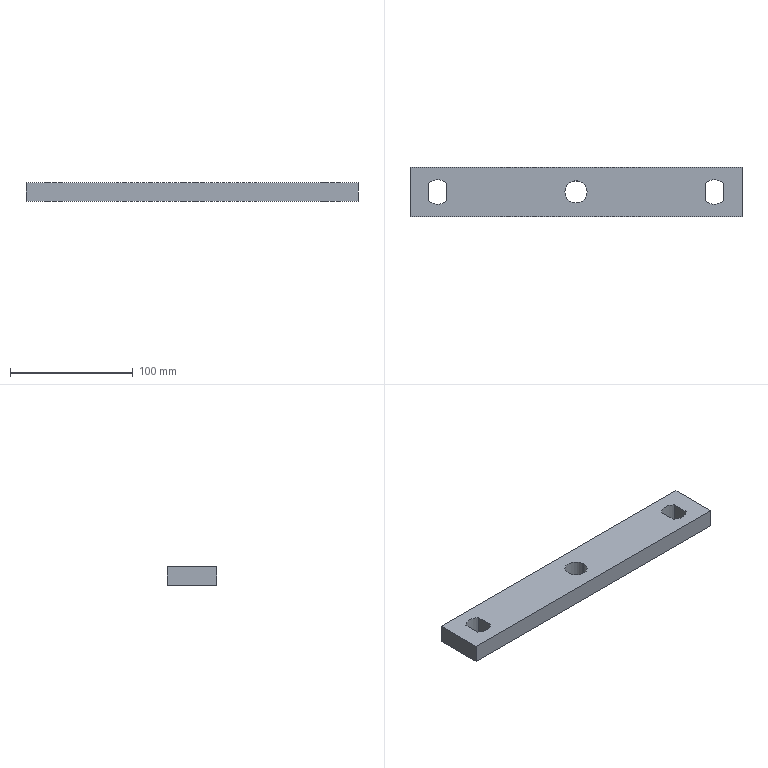Part | STEP file | Link hanger plate | 1 solid | 16 faces | box 270 x 40 x 15 mm | volume 150118 mm3 | plane 10 | cylinder 6 | commonest cylinder face diameters 20 x4 18 x2
STEP:
#1=CARTESIAN_POINT('',(0.,0.,0.));
#2=DIRECTION('',(0.,0.,1.));
#3=DIRECTION('',(1.,0.,0.));
#4=AXIS2_PLACEMENT_3D('',#1,#2,#3);
#5=CARTESIAN_POINT('',(9.,10.,-7.5));
#6=VERTEX_POINT('',#5);
#7=CARTESIAN_POINT('',(9.,10.,7.5));
#8=VERTEX_POINT('',#7);
#9=CARTESIAN_POINT('',(9.,10.,7.5));
#10=DIRECTION('',(0.,0.,1.));
#11=VECTOR('',#10,1.);
#12=LINE('',#9,#11);
#13=CARTESIAN_POINT('',(0.,10.,7.5));
#14=DIRECTION('',(0.,0.,1.));
#15=DIRECTION('',(1.,0.,0.));
#16=AXIS2_PLACEMENT_3D('',#13,#14,#15);
#17=CYLINDRICAL_SURFACE('',#16,9.);
#18=CARTESIAN_POINT('',(6.283,0.));
#19=DIRECTION('',(0.,1.));
#20=VECTOR('',#19,1.);
#21=LINE('',#18,#20);
#22=(GEOMETRIC_REPRESENTATION_CONTEXT(2)PARAMETRIC_REPRESENTATION_CONTEXT()REPRESENTATION_CONTEXT('',''));
#23=DEFINITIONAL_REPRESENTATION('',(#21),#22);
#24=PCURVE('',#17,#23);
#25=CARTESIAN_POINT('',(0.,10.,7.5));
#26=DIRECTION('',(0.,0.,1.));
#27=DIRECTION('',(1.,0.,0.));
#28=AXIS2_PLACEMENT_3D('',#25,#26,#27);
#29=CYLINDRICAL_SURFACE('',#28,9.);
#30=CARTESIAN_POINT('',(0.,0.));
#31=DIRECTION('',(0.,1.));
#32=VECTOR('',#31,1.);
#33=LINE('',#30,#32);
#34=(GEOMETRIC_REPRESENTATION_CONTEXT(2)PARAMETRIC_REPRESENTATION_CONTEXT()REPRESENTATION_CONTEXT('',''));
#35=DEFINITIONAL_REPRESENTATION('',(#33),#34);
#36=PCURVE('',#29,#35);
#37=SURFACE_CURVE('',#12,(#24,#36),.PCURVE_S1.);
#38=EDGE_CURVE('',#6,#8,#37,.T.);
#39=ORIENTED_EDGE('',*,*,#38,.T.);
#40=CARTESIAN_POINT('',(-9.,10.,7.5));
#41=VERTEX_POINT('',#40);
#42=CARTESIAN_POINT('',(0.,10.,7.5));
#43=DIRECTION('',(0.,0.,1.));
#44=DIRECTION('',(1.,0.,0.));
#45=AXIS2_PLACEMENT_3D('',#42,#43,#44);
#46=CIRCLE('',#45,9.);
#47=CARTESIAN_POINT('',(0.,0.));
#48=DIRECTION('',(1.,0.));
#49=VECTOR('',#48,1.);
#50=LINE('',#47,#49);
#51=(GEOMETRIC_REPRESENTATION_CONTEXT(2)PARAMETRIC_REPRESENTATION_CONTEXT()REPRESENTATION_CONTEXT('',''));
#52=DEFINITIONAL_REPRESENTATION('',(#50),#51);
#53=PCURVE('',#17,#52);
#54=CARTESIAN_POINT('',(0.,0.,7.5));
#55=DIRECTION('',(0.,0.,1.));
#56=DIRECTION('',(1.,0.,0.));
#57=AXIS2_PLACEMENT_3D('',#54,#55,#56);
#58=PLANE('',#57);
#59=CARTESIAN_POINT('',(0.,10.));
#60=DIRECTION('',(1.,0.));
#61=AXIS2_PLACEMENT_2D('',#59,#60);
#62=CIRCLE('',#61,9.);
#63=(GEOMETRIC_REPRESENTATION_CONTEXT(2)PARAMETRIC_REPRESENTATION_CONTEXT()REPRESENTATION_CONTEXT('',''));
#64=DEFINITIONAL_REPRESENTATION('',(#62),#63);
#65=PCURVE('',#58,#64);
#66=SURFACE_CURVE('',#46,(#53,#65),.PCURVE_S1.);
#67=EDGE_CURVE('',#41,#8,#66,.T.);
#68=ORIENTED_EDGE('',*,*,#67,.F.);
#69=CARTESIAN_POINT('',(-9.,10.,-7.5));
#70=VERTEX_POINT('',#69);
#71=CARTESIAN_POINT('',(-9.,10.,7.5));
#72=DIRECTION('',(0.,0.,1.));
#73=VECTOR('',#72,1.);
#74=LINE('',#71,#73);
#75=CARTESIAN_POINT('',(3.142,0.));
#76=DIRECTION('',(0.,1.));
#77=VECTOR('',#76,1.);
#78=LINE('',#75,#77);
#79=(GEOMETRIC_REPRESENTATION_CONTEXT(2)PARAMETRIC_REPRESENTATION_CONTEXT()REPRESENTATION_CONTEXT('',''));
#80=DEFINITIONAL_REPRESENTATION('',(#78),#79);
#81=PCURVE('',#17,#80);
#82=CARTESIAN_POINT('',(3.142,0.));
#83=DIRECTION('',(0.,1.));
#84=VECTOR('',#83,1.);
#85=LINE('',#82,#84);
#86=(GEOMETRIC_REPRESENTATION_CONTEXT(2)PARAMETRIC_REPRESENTATION_CONTEXT()REPRESENTATION_CONTEXT('',''));
#87=DEFINITIONAL_REPRESENTATION('',(#85),#86);
#88=PCURVE('',#29,#87);
#89=SURFACE_CURVE('',#74,(#81,#88),.PCURVE_S1.);
#90=EDGE_CURVE('',#70,#41,#89,.T.);
#91=ORIENTED_EDGE('',*,*,#90,.F.);
#92=CARTESIAN_POINT('',(0.,10.,-7.5));
#93=DIRECTION('',(0.,0.,1.));
#94=DIRECTION('',(1.,0.,0.));
#95=AXIS2_PLACEMENT_3D('',#92,#93,#94);
#96=CIRCLE('',#95,9.);
#97=CARTESIAN_POINT('',(0.,-15.));
#98=DIRECTION('',(1.,0.));
#99=VECTOR('',#98,1.);
#100=LINE('',#97,#99);
#101=(GEOMETRIC_REPRESENTATION_CONTEXT(2)PARAMETRIC_REPRESENTATION_CONTEXT()REPRESENTATION_CONTEXT('',''));
#102=DEFINITIONAL_REPRESENTATION('',(#100),#101);
#103=PCURVE('',#17,#102);
#104=CARTESIAN_POINT('',(0.,0.,-7.5));
#105=DIRECTION('',(0.,0.,1.));
#106=DIRECTION('',(1.,0.,0.));
#107=AXIS2_PLACEMENT_3D('',#104,#105,#106);
#108=PLANE('',#107);
#109=CARTESIAN_POINT('',(0.,10.));
#110=DIRECTION('',(1.,0.));
#111=AXIS2_PLACEMENT_2D('',#109,#110);
#112=CIRCLE('',#111,9.);
#113=(GEOMETRIC_REPRESENTATION_CONTEXT(2)PARAMETRIC_REPRESENTATION_CONTEXT()REPRESENTATION_CONTEXT('',''));
#114=DEFINITIONAL_REPRESENTATION('',(#112),#113);
#115=PCURVE('',#108,#114);
#116=SURFACE_CURVE('',#96,(#103,#115),.PCURVE_S1.);
#117=EDGE_CURVE('',#70,#6,#116,.T.);
#118=ORIENTED_EDGE('',*,*,#117,.T.);
#119=EDGE_LOOP('',(#39,#68,#91,#118));
#120=FACE_BOUND('',#119,.F.);
#121=ADVANCED_FACE('',(#120),#17,.F.);
#122=CARTESIAN_POINT('',(-135.,30.,7.5));
#123=VERTEX_POINT('',#122);
#124=CARTESIAN_POINT('',(-135.,-10.,7.5));
#125=VERTEX_POINT('',#124);
#126=CARTESIAN_POINT('',(-135.,30.,7.5));
#127=DIRECTION('',(0.,-1.,0.));
#128=VECTOR('',#127,1.);
#129=LINE('',#126,#128);
#130=CARTESIAN_POINT('',(-135.,30.));
#131=DIRECTION('',(0.,-1.));
#132=VECTOR('',#131,1.);
#133=LINE('',#130,#132);
#134=(GEOMETRIC_REPRESENTATION_CONTEXT(2)PARAMETRIC_REPRESENTATION_CONTEXT()REPRESENTATION_CONTEXT('',''));
#135=DEFINITIONAL_REPRESENTATION('',(#133),#134);
#136=PCURVE('',#58,#135);
#137=CARTESIAN_POINT('',(-135.,30.,7.5));
#138=DIRECTION('',(1.,0.,0.));
#139=DIRECTION('',(0.,0.,-1.));
#140=AXIS2_PLACEMENT_3D('',#137,#138,#139);
#141=PLANE('',#140);
#142=CARTESIAN_POINT('',(0.,0.));
#143=DIRECTION('',(0.,-1.));
#144=VECTOR('',#143,1.);
#145=LINE('',#142,#144);
#146=(GEOMETRIC_REPRESENTATION_CONTEXT(2)PARAMETRIC_REPRESENTATION_CONTEXT()REPRESENTATION_CONTEXT('',''));
#147=DEFINITIONAL_REPRESENTATION('',(#145),#146);
#148=PCURVE('',#141,#147);
#149=SURFACE_CURVE('',#129,(#136,#148),.PCURVE_S1.);
#150=EDGE_CURVE('',#123,#125,#149,.T.);
#151=ORIENTED_EDGE('',*,*,#150,.T.);
#152=CARTESIAN_POINT('',(135.,-10.,7.5));
#153=VERTEX_POINT('',#152);
#154=CARTESIAN_POINT('',(135.,-10.,7.5));
#155=DIRECTION('',(1.,0.,0.));
#156=VECTOR('',#155,1.);
#157=LINE('',#154,#156);
#158=CARTESIAN_POINT('',(135.,-10.));
#159=DIRECTION('',(1.,0.));
#160=VECTOR('',#159,1.);
#161=LINE('',#158,#160);
#162=(GEOMETRIC_REPRESENTATION_CONTEXT(2)PARAMETRIC_REPRESENTATION_CONTEXT()REPRESENTATION_CONTEXT('',''));
#163=DEFINITIONAL_REPRESENTATION('',(#161),#162);
#164=PCURVE('',#58,#163);
#165=CARTESIAN_POINT('',(135.,-10.,7.5));
#166=DIRECTION('',(0.,1.,0.));
#167=DIRECTION('',(0.,0.,1.));
#168=AXIS2_PLACEMENT_3D('',#165,#166,#167);
#169=PLANE('',#168);
#170=CARTESIAN_POINT('',(0.,0.));
#171=DIRECTION('',(0.,1.));
#172=VECTOR('',#171,1.);
#173=LINE('',#170,#172);
#174=(GEOMETRIC_REPRESENTATION_CONTEXT(2)PARAMETRIC_REPRESENTATION_CONTEXT()REPRESENTATION_CONTEXT('',''));
#175=DEFINITIONAL_REPRESENTATION('',(#173),#174);
#176=PCURVE('',#169,#175);
#177=SURFACE_CURVE('',#157,(#164,#176),.PCURVE_S1.);
#178=EDGE_CURVE('',#125,#153,#177,.T.);
#179=ORIENTED_EDGE('',*,*,#178,.T.);
#180=CARTESIAN_POINT('',(135.,30.,7.5));
#181=VERTEX_POINT('',#180);
#182=CARTESIAN_POINT('',(135.,30.,7.5));
#183=DIRECTION('',(0.,1.,0.));
#184=VECTOR('',#183,1.);
#185=LINE('',#182,#184);
#186=CARTESIAN_POINT('',(135.,30.));
#187=DIRECTION('',(0.,1.));
#188=VECTOR('',#187,1.);
#189=LINE('',#186,#188);
#190=(GEOMETRIC_REPRESENTATION_CONTEXT(2)PARAMETRIC_REPRESENTATION_CONTEXT()REPRESENTATION_CONTEXT('',''));
#191=DEFINITIONAL_REPRESENTATION('',(#189),#190);
#192=PCURVE('',#58,#191);
#193=CARTESIAN_POINT('',(135.,30.,7.5));
#194=DIRECTION('',(-1.,0.,0.));
#195=DIRECTION('',(0.,-1.,0.));
#196=AXIS2_PLACEMENT_3D('',#193,#194,#195);
#197=PLANE('',#196);
#198=CARTESIAN_POINT('',(0.,0.));
#199=DIRECTION('',(-1.,0.));
#200=VECTOR('',#199,1.);
#201=LINE('',#198,#200);
#202=(GEOMETRIC_REPRESENTATION_CONTEXT(2)PARAMETRIC_REPRESENTATION_CONTEXT()REPRESENTATION_CONTEXT('',''));
#203=DEFINITIONAL_REPRESENTATION('',(#201),#202);
#204=PCURVE('',#197,#203);
#205=SURFACE_CURVE('',#185,(#192,#204),.PCURVE_S1.);
#206=EDGE_CURVE('',#153,#181,#205,.T.);
#207=ORIENTED_EDGE('',*,*,#206,.T.);
#208=CARTESIAN_POINT('',(-135.,30.,7.5));
#209=DIRECTION('',(-1.,0.,0.));
#210=VECTOR('',#209,1.);
#211=LINE('',#208,#210);
#212=CARTESIAN_POINT('',(-135.,30.));
#213=DIRECTION('',(-1.,0.));
#214=VECTOR('',#213,1.);
#215=LINE('',#212,#214);
#216=(GEOMETRIC_REPRESENTATION_CONTEXT(2)PARAMETRIC_REPRESENTATION_CONTEXT()REPRESENTATION_CONTEXT('',''));
#217=DEFINITIONAL_REPRESENTATION('',(#215),#216);
#218=PCURVE('',#58,#217);
#219=CARTESIAN_POINT('',(-135.,30.,7.5));
#220=DIRECTION('',(0.,-1.,0.));
#221=DIRECTION('',(0.,0.,-1.));
#222=AXIS2_PLACEMENT_3D('',#219,#220,#221);
#223=PLANE('',#222);
#224=CARTESIAN_POINT('',(0.,0.));
#225=DIRECTION('',(0.,-1.));
#226=VECTOR('',#225,1.);
#227=LINE('',#224,#226);
#228=(GEOMETRIC_REPRESENTATION_CONTEXT(2)PARAMETRIC_REPRESENTATION_CONTEXT()REPRESENTATION_CONTEXT('',''));
#229=DEFINITIONAL_REPRESENTATION('',(#227),#228);
#230=PCURVE('',#223,#229);
#231=SURFACE_CURVE('',#211,(#218,#230),.PCURVE_S1.);
#232=EDGE_CURVE('',#181,#123,#231,.T.);
#233=ORIENTED_EDGE('',*,*,#232,.T.);
#234=EDGE_LOOP('',(#151,#179,#207,#233));
#235=FACE_BOUND('',#234,.T.);
#236=CARTESIAN_POINT('',(120.,16.614,7.5));
#237=VERTEX_POINT('',#236);
#238=CARTESIAN_POINT('',(120.,3.386,7.5));
#239=VERTEX_POINT('',#238);
#240=CARTESIAN_POINT('',(120.,16.614,7.5));
#241=DIRECTION('',(0.,-1.,0.));
#242=VECTOR('',#241,1.);
#243=LINE('',#240,#242);
#244=CARTESIAN_POINT('',(120.,16.614));
#245=DIRECTION('',(0.,-1.));
#246=VECTOR('',#245,1.);
#247=LINE('',#244,#246);
#248=(GEOMETRIC_REPRESENTATION_CONTEXT(2)PARAMETRIC_REPRESENTATION_CONTEXT()REPRESENTATION_CONTEXT('',''));
#249=DEFINITIONAL_REPRESENTATION('',(#247),#248);
#250=PCURVE('',#58,#249);
#251=CARTESIAN_POINT('',(120.,16.614,-7.5));
#252=DIRECTION('',(-1.,0.,0.));
#253=DIRECTION('',(0.,0.,1.));
#254=AXIS2_PLACEMENT_3D('',#251,#252,#253);
#255=PLANE('',#254);
#256=CARTESIAN_POINT('',(15.,0.));
#257=DIRECTION('',(0.,-1.));
#258=VECTOR('',#257,1.);
#259=LINE('',#256,#258);
#260=(GEOMETRIC_REPRESENTATION_CONTEXT(2)PARAMETRIC_REPRESENTATION_CONTEXT()REPRESENTATION_CONTEXT('',''));
#261=DEFINITIONAL_REPRESENTATION('',(#259),#260);
#262=PCURVE('',#255,#261);
#263=SURFACE_CURVE('',#243,(#250,#262),.PCURVE_S1.);
#264=EDGE_CURVE('',#237,#239,#263,.T.);
#265=ORIENTED_EDGE('',*,*,#264,.T.);
#266=CARTESIAN_POINT('',(105.,3.386,7.5));
#267=VERTEX_POINT('',#266);
#268=CARTESIAN_POINT('',(112.5,10.,7.5));
#269=DIRECTION('',(0.,0.,-1.));
#270=DIRECTION('',(-1.,0.,0.));
#271=AXIS2_PLACEMENT_3D('',#268,#269,#270);
#272=CIRCLE('',#271,10.);
#273=CARTESIAN_POINT('',(102.5,10.));
#274=CARTESIAN_POINT('',(102.5,27.321));
#275=CARTESIAN_POINT('',(117.5,18.66));
#276=CARTESIAN_POINT('',(132.5,10.));
#277=CARTESIAN_POINT('',(117.5,1.34));
#278=CARTESIAN_POINT('',(102.5,-7.321));
#279=CARTESIAN_POINT('',(102.5,10.));
#280=(BOUNDED_CURVE()B_SPLINE_CURVE(2,(#273,#274,#275,#276,#277,#278,#279),.UNSPECIFIED.,.T.,.F.)B_SPLINE_CURVE_WITH_KNOTS((1,2,2,2,2,1),(-2.094,0.,2.094,4.189,6.283,8.378),.UNSPECIFIED.)CURVE()GEOMETRIC_REPRESENTATION_ITEM()RATIONAL_B_SPLINE_CURVE((1.,0.5,1.,0.5,1.,0.5,1.))REPRESENTATION_ITEM(''));
#281=(GEOMETRIC_REPRESENTATION_CONTEXT(2)PARAMETRIC_REPRESENTATION_CONTEXT()REPRESENTATION_CONTEXT('',''));
#282=DEFINITIONAL_REPRESENTATION('',(#280),#281);
#283=PCURVE('',#58,#282);
#284=CARTESIAN_POINT('',(112.5,10.,-7.5));
#285=DIRECTION('',(0.,0.,1.));
#286=DIRECTION('',(1.,0.,0.));
#287=AXIS2_PLACEMENT_3D('',#284,#285,#286);
#288=CYLINDRICAL_SURFACE('',#287,10.);
#289=CARTESIAN_POINT('',(9.425,15.));
#290=DIRECTION('',(-1.,0.));
#291=VECTOR('',#290,1.);
#292=LINE('',#289,#291);
#293=(GEOMETRIC_REPRESENTATION_CONTEXT(2)PARAMETRIC_REPRESENTATION_CONTEXT()REPRESENTATION_CONTEXT('',''));
#294=DEFINITIONAL_REPRESENTATION('',(#292),#293);
#295=PCURVE('',#288,#294);
#296=SURFACE_CURVE('',#272,(#283,#295),.PCURVE_S1.);
#297=EDGE_CURVE('',#239,#267,#296,.T.);
#298=ORIENTED_EDGE('',*,*,#297,.T.);
#299=CARTESIAN_POINT('',(105.,16.614,7.5));
#300=VERTEX_POINT('',#299);
#301=CARTESIAN_POINT('',(105.,16.614,7.5));
#302=DIRECTION('',(0.,1.,0.));
#303=VECTOR('',#302,1.);
#304=LINE('',#301,#303);
#305=CARTESIAN_POINT('',(105.,16.614));
#306=DIRECTION('',(0.,1.));
#307=VECTOR('',#306,1.);
#308=LINE('',#305,#307);
#309=(GEOMETRIC_REPRESENTATION_CONTEXT(2)PARAMETRIC_REPRESENTATION_CONTEXT()REPRESENTATION_CONTEXT('',''));
#310=DEFINITIONAL_REPRESENTATION('',(#308),#309);
#311=PCURVE('',#58,#310);
#312=CARTESIAN_POINT('',(105.,16.614,-7.5));
#313=DIRECTION('',(1.,0.,0.));
#314=DIRECTION('',(0.,0.,-1.));
#315=AXIS2_PLACEMENT_3D('',#312,#313,#314);
#316=PLANE('',#315);
#317=CARTESIAN_POINT('',(-15.,0.));
#318=DIRECTION('',(0.,1.));
#319=VECTOR('',#318,1.);
#320=LINE('',#317,#319);
#321=(GEOMETRIC_REPRESENTATION_CONTEXT(2)PARAMETRIC_REPRESENTATION_CONTEXT()REPRESENTATION_CONTEXT('',''));
#322=DEFINITIONAL_REPRESENTATION('',(#320),#321);
#323=PCURVE('',#316,#322);
#324=SURFACE_CURVE('',#304,(#311,#323),.PCURVE_S1.);
#325=EDGE_CURVE('',#267,#300,#324,.T.);
#326=ORIENTED_EDGE('',*,*,#325,.T.);
#327=CARTESIAN_POINT('',(112.5,10.,7.5));
#328=DIRECTION('',(0.,0.,-1.));
#329=DIRECTION('',(-1.,0.,0.));
#330=AXIS2_PLACEMENT_3D('',#327,#328,#329);
#331=CIRCLE('',#330,10.);
#332=CARTESIAN_POINT('',(102.5,10.));
#333=CARTESIAN_POINT('',(102.5,27.321));
#334=CARTESIAN_POINT('',(117.5,18.66));
#335=CARTESIAN_POINT('',(132.5,10.));
#336=CARTESIAN_POINT('',(117.5,1.34));
#337=CARTESIAN_POINT('',(102.5,-7.321));
#338=CARTESIAN_POINT('',(102.5,10.));
#339=(BOUNDED_CURVE()B_SPLINE_CURVE(2,(#332,#333,#334,#335,#336,#337,#338),.UNSPECIFIED.,.T.,.F.)B_SPLINE_CURVE_WITH_KNOTS((1,2,2,2,2,1),(-2.094,0.,2.094,4.189,6.283,8.378),.UNSPECIFIED.)CURVE()GEOMETRIC_REPRESENTATION_ITEM()RATIONAL_B_SPLINE_CURVE((1.,0.5,1.,0.5,1.,0.5,1.))REPRESENTATION_ITEM(''));
#340=(GEOMETRIC_REPRESENTATION_CONTEXT(2)PARAMETRIC_REPRESENTATION_CONTEXT()REPRESENTATION_CONTEXT('',''));
#341=DEFINITIONAL_REPRESENTATION('',(#339),#340);
#342=PCURVE('',#58,#341);
#343=CARTESIAN_POINT('',(112.5,10.,-7.5));
#344=DIRECTION('',(0.,0.,1.));
#345=DIRECTION('',(1.,0.,0.));
#346=AXIS2_PLACEMENT_3D('',#343,#344,#345);
#347=CYLINDRICAL_SURFACE('',#346,10.);
#348=CARTESIAN_POINT('',(3.142,15.));
#349=DIRECTION('',(-1.,0.));
#350=VECTOR('',#349,1.);
#351=LINE('',#348,#350);
#352=(GEOMETRIC_REPRESENTATION_CONTEXT(2)PARAMETRIC_REPRESENTATION_CONTEXT()REPRESENTATION_CONTEXT('',''));
#353=DEFINITIONAL_REPRESENTATION('',(#351),#352);
#354=PCURVE('',#347,#353);
#355=SURFACE_CURVE('',#331,(#342,#354),.PCURVE_S1.);
#356=EDGE_CURVE('',#300,#237,#355,.T.);
#357=ORIENTED_EDGE('',*,*,#356,.T.);
#358=EDGE_LOOP('',(#265,#298,#326,#357));
#359=FACE_BOUND('',#358,.T.);
#360=CARTESIAN_POINT('',(-120.,3.386,7.5));
#361=VERTEX_POINT('',#360);
#362=CARTESIAN_POINT('',(-105.,3.386,7.5));
#363=VERTEX_POINT('',#362);
#364=CARTESIAN_POINT('',(-112.5,10.,7.5));
#365=DIRECTION('',(0.,0.,1.));
#366=DIRECTION('',(1.,0.,0.));
#367=AXIS2_PLACEMENT_3D('',#364,#365,#366);
#368=CIRCLE('',#367,10.);
#369=CARTESIAN_POINT('',(-112.5,10.));
#370=DIRECTION('',(1.,0.));
#371=AXIS2_PLACEMENT_2D('',#369,#370);
#372=CIRCLE('',#371,10.);
#373=(GEOMETRIC_REPRESENTATION_CONTEXT(2)PARAMETRIC_REPRESENTATION_CONTEXT()REPRESENTATION_CONTEXT('',''));
#374=DEFINITIONAL_REPRESENTATION('',(#372),#373);
#375=PCURVE('',#58,#374);
#376=CARTESIAN_POINT('',(-112.5,10.,-7.5));
#377=DIRECTION('',(0.,0.,1.));
#378=DIRECTION('',(1.,0.,0.));
#379=AXIS2_PLACEMENT_3D('',#376,#377,#378);
#380=CYLINDRICAL_SURFACE('',#379,10.);
#381=CARTESIAN_POINT('',(0.,15.));
#382=DIRECTION('',(1.,0.));
#383=VECTOR('',#382,1.);
#384=LINE('',#381,#383);
#385=(GEOMETRIC_REPRESENTATION_CONTEXT(2)PARAMETRIC_REPRESENTATION_CONTEXT()REPRESENTATION_CONTEXT('',''));
#386=DEFINITIONAL_REPRESENTATION('',(#384),#385);
#387=PCURVE('',#380,#386);
#388=SURFACE_CURVE('',#368,(#375,#387),.PCURVE_S1.);
#389=EDGE_CURVE('',#361,#363,#388,.T.);
#390=ORIENTED_EDGE('',*,*,#389,.F.);
#391=CARTESIAN_POINT('',(-120.,16.614,7.5));
#392=VERTEX_POINT('',#391);
#393=CARTESIAN_POINT('',(-120.,16.614,7.5));
#394=DIRECTION('',(0.,-1.,0.));
#395=VECTOR('',#394,1.);
#396=LINE('',#393,#395);
#397=CARTESIAN_POINT('',(-120.,16.614));
#398=DIRECTION('',(0.,-1.));
#399=VECTOR('',#398,1.);
#400=LINE('',#397,#399);
#401=(GEOMETRIC_REPRESENTATION_CONTEXT(2)PARAMETRIC_REPRESENTATION_CONTEXT()REPRESENTATION_CONTEXT('',''));
#402=DEFINITIONAL_REPRESENTATION('',(#400),#401);
#403=PCURVE('',#58,#402);
#404=CARTESIAN_POINT('',(-120.,16.614,-7.5));
#405=DIRECTION('',(-1.,0.,0.));
#406=DIRECTION('',(0.,0.,1.));
#407=AXIS2_PLACEMENT_3D('',#404,#405,#406);
#408=PLANE('',#407);
#409=CARTESIAN_POINT('',(15.,0.));
#410=DIRECTION('',(0.,-1.));
#411=VECTOR('',#410,1.);
#412=LINE('',#409,#411);
#413=(GEOMETRIC_REPRESENTATION_CONTEXT(2)PARAMETRIC_REPRESENTATION_CONTEXT()REPRESENTATION_CONTEXT('',''));
#414=DEFINITIONAL_REPRESENTATION('',(#412),#413);
#415=PCURVE('',#408,#414);
#416=SURFACE_CURVE('',#396,(#403,#415),.PCURVE_S1.);
#417=EDGE_CURVE('',#392,#361,#416,.T.);
#418=ORIENTED_EDGE('',*,*,#417,.F.);
#419=CARTESIAN_POINT('',(-105.,16.614,7.5));
#420=VERTEX_POINT('',#419);
#421=CARTESIAN_POINT('',(-112.5,10.,7.5));
#422=DIRECTION('',(0.,0.,1.));
#423=DIRECTION('',(1.,0.,0.));
#424=AXIS2_PLACEMENT_3D('',#421,#422,#423);
#425=CIRCLE('',#424,10.);
#426=CARTESIAN_POINT('',(-112.5,10.));
#427=DIRECTION('',(1.,0.));
#428=AXIS2_PLACEMENT_2D('',#426,#427);
#429=CIRCLE('',#428,10.);
#430=(GEOMETRIC_REPRESENTATION_CONTEXT(2)PARAMETRIC_REPRESENTATION_CONTEXT()REPRESENTATION_CONTEXT('',''));
#431=DEFINITIONAL_REPRESENTATION('',(#429),#430);
#432=PCURVE('',#58,#431);
#433=CARTESIAN_POINT('',(-112.5,10.,-7.5));
#434=DIRECTION('',(0.,0.,1.));
#435=DIRECTION('',(1.,0.,0.));
#436=AXIS2_PLACEMENT_3D('',#433,#434,#435);
#437=CYLINDRICAL_SURFACE('',#436,10.);
#438=CARTESIAN_POINT('',(0.,15.));
#439=DIRECTION('',(1.,0.));
#440=VECTOR('',#439,1.);
#441=LINE('',#438,#440);
#442=(GEOMETRIC_REPRESENTATION_CONTEXT(2)PARAMETRIC_REPRESENTATION_CONTEXT()REPRESENTATION_CONTEXT('',''));
#443=DEFINITIONAL_REPRESENTATION('',(#441),#442);
#444=PCURVE('',#437,#443);
#445=SURFACE_CURVE('',#425,(#432,#444),.PCURVE_S1.);
#446=EDGE_CURVE('',#420,#392,#445,.T.);
#447=ORIENTED_EDGE('',*,*,#446,.F.);
#448=CARTESIAN_POINT('',(-105.,16.614,7.5));
#449=DIRECTION('',(0.,1.,0.));
#450=VECTOR('',#449,1.);
#451=LINE('',#448,#450);
#452=CARTESIAN_POINT('',(-105.,16.614));
#453=DIRECTION('',(0.,1.));
#454=VECTOR('',#453,1.);
#455=LINE('',#452,#454);
#456=(GEOMETRIC_REPRESENTATION_CONTEXT(2)PARAMETRIC_REPRESENTATION_CONTEXT()REPRESENTATION_CONTEXT('',''));
#457=DEFINITIONAL_REPRESENTATION('',(#455),#456);
#458=PCURVE('',#58,#457);
#459=CARTESIAN_POINT('',(-105.,16.614,-7.5));
#460=DIRECTION('',(1.,0.,0.));
#461=DIRECTION('',(0.,0.,-1.));
#462=AXIS2_PLACEMENT_3D('',#459,#460,#461);
#463=PLANE('',#462);
#464=CARTESIAN_POINT('',(-15.,0.));
#465=DIRECTION('',(0.,1.));
#466=VECTOR('',#465,1.);
#467=LINE('',#464,#466);
#468=(GEOMETRIC_REPRESENTATION_CONTEXT(2)PARAMETRIC_REPRESENTATION_CONTEXT()REPRESENTATION_CONTEXT('',''));
#469=DEFINITIONAL_REPRESENTATION('',(#467),#468);
#470=PCURVE('',#463,#469);
#471=SURFACE_CURVE('',#451,(#458,#470),.PCURVE_S1.);
#472=EDGE_CURVE('',#363,#420,#471,.T.);
#473=ORIENTED_EDGE('',*,*,#472,.F.);
#474=EDGE_LOOP('',(#390,#418,#447,#473));
#475=FACE_BOUND('',#474,.T.);
#476=CARTESIAN_POINT('',(0.,10.,7.5));
#477=DIRECTION('',(0.,0.,1.));
#478=DIRECTION('',(1.,0.,0.));
#479=AXIS2_PLACEMENT_3D('',#476,#477,#478);
#480=CIRCLE('',#479,9.);
#481=CARTESIAN_POINT('',(0.,10.));
#482=DIRECTION('',(1.,0.));
#483=AXIS2_PLACEMENT_2D('',#481,#482);
#484=CIRCLE('',#483,9.);
#485=(GEOMETRIC_REPRESENTATION_CONTEXT(2)PARAMETRIC_REPRESENTATION_CONTEXT()REPRESENTATION_CONTEXT('',''));
#486=DEFINITIONAL_REPRESENTATION('',(#484),#485);
#487=PCURVE('',#58,#486);
#488=CARTESIAN_POINT('',(0.,0.));
#489=DIRECTION('',(1.,0.));
#490=VECTOR('',#489,1.);
#491=LINE('',#488,#490);
#492=(GEOMETRIC_REPRESENTATION_CONTEXT(2)PARAMETRIC_REPRESENTATION_CONTEXT()REPRESENTATION_CONTEXT('',''));
#493=DEFINITIONAL_REPRESENTATION('',(#491),#492);
#494=PCURVE('',#29,#493);
#495=SURFACE_CURVE('',#480,(#487,#494),.PCURVE_S1.);
#496=EDGE_CURVE('',#8,#41,#495,.T.);
#497=ORIENTED_EDGE('',*,*,#496,.F.);
#498=ORIENTED_EDGE('',*,*,#67,.F.);
#499=EDGE_LOOP('',(#497,#498));
#500=FACE_BOUND('',#499,.T.);
#501=ADVANCED_FACE('',(#235,#359,#475,#500),#58,.T.);
#502=CARTESIAN_POINT('',(120.,3.386,-7.5));
#503=VERTEX_POINT('',#502);
#504=CARTESIAN_POINT('',(105.,3.386,-7.5));
#505=VERTEX_POINT('',#504);
#506=CARTESIAN_POINT('',(112.5,10.,-7.5));
#507=DIRECTION('',(0.,0.,-1.));
#508=DIRECTION('',(-1.,0.,0.));
#509=AXIS2_PLACEMENT_3D('',#506,#507,#508);
#510=CIRCLE('',#509,10.);
#511=CARTESIAN_POINT('',(102.5,10.));
#512=CARTESIAN_POINT('',(102.5,27.321));
#513=CARTESIAN_POINT('',(117.5,18.66));
#514=CARTESIAN_POINT('',(132.5,10.));
#515=CARTESIAN_POINT('',(117.5,1.34));
#516=CARTESIAN_POINT('',(102.5,-7.321));
#517=CARTESIAN_POINT('',(102.5,10.));
#518=(BOUNDED_CURVE()B_SPLINE_CURVE(2,(#511,#512,#513,#514,#515,#516,#517),.UNSPECIFIED.,.T.,.F.)B_SPLINE_CURVE_WITH_KNOTS((1,2,2,2,2,1),(-2.094,0.,2.094,4.189,6.283,8.378),.UNSPECIFIED.)CURVE()GEOMETRIC_REPRESENTATION_ITEM()RATIONAL_B_SPLINE_CURVE((1.,0.5,1.,0.5,1.,0.5,1.))REPRESENTATION_ITEM(''));
#519=(GEOMETRIC_REPRESENTATION_CONTEXT(2)PARAMETRIC_REPRESENTATION_CONTEXT()REPRESENTATION_CONTEXT('',''));
#520=DEFINITIONAL_REPRESENTATION('',(#518),#519);
#521=PCURVE('',#108,#520);
#522=CARTESIAN_POINT('',(9.425,0.));
#523=DIRECTION('',(-1.,0.));
#524=VECTOR('',#523,1.);
#525=LINE('',#522,#524);
#526=(GEOMETRIC_REPRESENTATION_CONTEXT(2)PARAMETRIC_REPRESENTATION_CONTEXT()REPRESENTATION_CONTEXT('',''));
#527=DEFINITIONAL_REPRESENTATION('',(#525),#526);
#528=PCURVE('',#288,#527);
#529=SURFACE_CURVE('',#510,(#521,#528),.PCURVE_S1.);
#530=EDGE_CURVE('',#503,#505,#529,.T.);
#531=ORIENTED_EDGE('',*,*,#530,.F.);
#532=CARTESIAN_POINT('',(120.,16.614,-7.5));
#533=VERTEX_POINT('',#532);
#534=CARTESIAN_POINT('',(120.,16.614,-7.5));
#535=DIRECTION('',(0.,-1.,0.));
#536=VECTOR('',#535,1.);
#537=LINE('',#534,#536);
#538=CARTESIAN_POINT('',(120.,16.614));
#539=DIRECTION('',(0.,-1.));
#540=VECTOR('',#539,1.);
#541=LINE('',#538,#540);
#542=(GEOMETRIC_REPRESENTATION_CONTEXT(2)PARAMETRIC_REPRESENTATION_CONTEXT()REPRESENTATION_CONTEXT('',''));
#543=DEFINITIONAL_REPRESENTATION('',(#541),#542);
#544=PCURVE('',#108,#543);
#545=CARTESIAN_POINT('',(0.,0.));
#546=DIRECTION('',(0.,-1.));
#547=VECTOR('',#546,1.);
#548=LINE('',#545,#547);
#549=(GEOMETRIC_REPRESENTATION_CONTEXT(2)PARAMETRIC_REPRESENTATION_CONTEXT()REPRESENTATION_CONTEXT('',''));
#550=DEFINITIONAL_REPRESENTATION('',(#548),#549);
#551=PCURVE('',#255,#550);
#552=SURFACE_CURVE('',#537,(#544,#551),.PCURVE_S1.);
#553=EDGE_CURVE('',#533,#503,#552,.T.);
#554=ORIENTED_EDGE('',*,*,#553,.F.);
#555=CARTESIAN_POINT('',(105.,16.614,-7.5));
#556=VERTEX_POINT('',#555);
#557=CARTESIAN_POINT('',(112.5,10.,-7.5));
#558=DIRECTION('',(0.,0.,-1.));
#559=DIRECTION('',(-1.,0.,0.));
#560=AXIS2_PLACEMENT_3D('',#557,#558,#559);
#561=CIRCLE('',#560,10.);
#562=CARTESIAN_POINT('',(102.5,10.));
#563=CARTESIAN_POINT('',(102.5,27.321));
#564=CARTESIAN_POINT('',(117.5,18.66));
#565=CARTESIAN_POINT('',(132.5,10.));
#566=CARTESIAN_POINT('',(117.5,1.34));
#567=CARTESIAN_POINT('',(102.5,-7.321));
#568=CARTESIAN_POINT('',(102.5,10.));
#569=(BOUNDED_CURVE()B_SPLINE_CURVE(2,(#562,#563,#564,#565,#566,#567,#568),.UNSPECIFIED.,.T.,.F.)B_SPLINE_CURVE_WITH_KNOTS((1,2,2,2,2,1),(-2.094,0.,2.094,4.189,6.283,8.378),.UNSPECIFIED.)CURVE()GEOMETRIC_REPRESENTATION_ITEM()RATIONAL_B_SPLINE_CURVE((1.,0.5,1.,0.5,1.,0.5,1.))REPRESENTATION_ITEM(''));
#570=(GEOMETRIC_REPRESENTATION_CONTEXT(2)PARAMETRIC_REPRESENTATION_CONTEXT()REPRESENTATION_CONTEXT('',''));
#571=DEFINITIONAL_REPRESENTATION('',(#569),#570);
#572=PCURVE('',#108,#571);
#573=CARTESIAN_POINT('',(3.142,0.));
#574=DIRECTION('',(-1.,0.));
#575=VECTOR('',#574,1.);
#576=LINE('',#573,#575);
#577=(GEOMETRIC_REPRESENTATION_CONTEXT(2)PARAMETRIC_REPRESENTATION_CONTEXT()REPRESENTATION_CONTEXT('',''));
#578=DEFINITIONAL_REPRESENTATION('',(#576),#577);
#579=PCURVE('',#347,#578);
#580=SURFACE_CURVE('',#561,(#572,#579),.PCURVE_S1.);
#581=EDGE_CURVE('',#556,#533,#580,.T.);
#582=ORIENTED_EDGE('',*,*,#581,.F.);
#583=CARTESIAN_POINT('',(105.,16.614,-7.5));
#584=DIRECTION('',(0.,1.,0.));
#585=VECTOR('',#584,1.);
#586=LINE('',#583,#585);
#587=CARTESIAN_POINT('',(105.,16.614));
#588=DIRECTION('',(0.,1.));
#589=VECTOR('',#588,1.);
#590=LINE('',#587,#589);
#591=(GEOMETRIC_REPRESENTATION_CONTEXT(2)PARAMETRIC_REPRESENTATION_CONTEXT()REPRESENTATION_CONTEXT('',''));
#592=DEFINITIONAL_REPRESENTATION('',(#590),#591);
#593=PCURVE('',#108,#592);
#594=CARTESIAN_POINT('',(0.,0.));
#595=DIRECTION('',(0.,1.));
#596=VECTOR('',#595,1.);
#597=LINE('',#594,#596);
#598=(GEOMETRIC_REPRESENTATION_CONTEXT(2)PARAMETRIC_REPRESENTATION_CONTEXT()REPRESENTATION_CONTEXT('',''));
#599=DEFINITIONAL_REPRESENTATION('',(#597),#598);
#600=PCURVE('',#316,#599);
#601=SURFACE_CURVE('',#586,(#593,#600),.PCURVE_S1.);
#602=EDGE_CURVE('',#505,#556,#601,.T.);
#603=ORIENTED_EDGE('',*,*,#602,.F.);
#604=EDGE_LOOP('',(#531,#554,#582,#603));
#605=FACE_BOUND('',#604,.T.);
#606=CARTESIAN_POINT('',(-120.,16.614,-7.5));
#607=VERTEX_POINT('',#606);
#608=CARTESIAN_POINT('',(-120.,3.386,-7.5));
#609=VERTEX_POINT('',#608);
#610=CARTESIAN_POINT('',(-120.,16.614,-7.5));
#611=DIRECTION('',(0.,-1.,0.));
#612=VECTOR('',#611,1.);
#613=LINE('',#610,#612);
#614=CARTESIAN_POINT('',(-120.,16.614));
#615=DIRECTION('',(0.,-1.));
#616=VECTOR('',#615,1.);
#617=LINE('',#614,#616);
#618=(GEOMETRIC_REPRESENTATION_CONTEXT(2)PARAMETRIC_REPRESENTATION_CONTEXT()REPRESENTATION_CONTEXT('',''));
#619=DEFINITIONAL_REPRESENTATION('',(#617),#618);
#620=PCURVE('',#108,#619);
#621=CARTESIAN_POINT('',(0.,0.));
#622=DIRECTION('',(0.,-1.));
#623=VECTOR('',#622,1.);
#624=LINE('',#621,#623);
#625=(GEOMETRIC_REPRESENTATION_CONTEXT(2)PARAMETRIC_REPRESENTATION_CONTEXT()REPRESENTATION_CONTEXT('',''));
#626=DEFINITIONAL_REPRESENTATION('',(#624),#625);
#627=PCURVE('',#408,#626);
#628=SURFACE_CURVE('',#613,(#620,#627),.PCURVE_S1.);
#629=EDGE_CURVE('',#607,#609,#628,.T.);
#630=ORIENTED_EDGE('',*,*,#629,.T.);
#631=CARTESIAN_POINT('',(-105.,3.386,-7.5));
#632=VERTEX_POINT('',#631);
#633=CARTESIAN_POINT('',(-112.5,10.,-7.5));
#634=DIRECTION('',(0.,0.,1.));
#635=DIRECTION('',(1.,0.,0.));
#636=AXIS2_PLACEMENT_3D('',#633,#634,#635);
#637=CIRCLE('',#636,10.);
#638=CARTESIAN_POINT('',(-112.5,10.));
#639=DIRECTION('',(1.,0.));
#640=AXIS2_PLACEMENT_2D('',#638,#639);
#641=CIRCLE('',#640,10.);
#642=(GEOMETRIC_REPRESENTATION_CONTEXT(2)PARAMETRIC_REPRESENTATION_CONTEXT()REPRESENTATION_CONTEXT('',''));
#643=DEFINITIONAL_REPRESENTATION('',(#641),#642);
#644=PCURVE('',#108,#643);
#645=CARTESIAN_POINT('',(0.,0.));
#646=DIRECTION('',(1.,0.));
#647=VECTOR('',#646,1.);
#648=LINE('',#645,#647);
#649=(GEOMETRIC_REPRESENTATION_CONTEXT(2)PARAMETRIC_REPRESENTATION_CONTEXT()REPRESENTATION_CONTEXT('',''));
#650=DEFINITIONAL_REPRESENTATION('',(#648),#649);
#651=PCURVE('',#380,#650);
#652=SURFACE_CURVE('',#637,(#644,#651),.PCURVE_S1.);
#653=EDGE_CURVE('',#609,#632,#652,.T.);
#654=ORIENTED_EDGE('',*,*,#653,.T.);
#655=CARTESIAN_POINT('',(-105.,16.614,-7.5));
#656=VERTEX_POINT('',#655);
#657=CARTESIAN_POINT('',(-105.,16.614,-7.5));
#658=DIRECTION('',(0.,1.,0.));
#659=VECTOR('',#658,1.);
#660=LINE('',#657,#659);
#661=CARTESIAN_POINT('',(-105.,16.614));
#662=DIRECTION('',(0.,1.));
#663=VECTOR('',#662,1.);
#664=LINE('',#661,#663);
#665=(GEOMETRIC_REPRESENTATION_CONTEXT(2)PARAMETRIC_REPRESENTATION_CONTEXT()REPRESENTATION_CONTEXT('',''));
#666=DEFINITIONAL_REPRESENTATION('',(#664),#665);
#667=PCURVE('',#108,#666);
#668=CARTESIAN_POINT('',(0.,0.));
#669=DIRECTION('',(0.,1.));
#670=VECTOR('',#669,1.);
#671=LINE('',#668,#670);
#672=(GEOMETRIC_REPRESENTATION_CONTEXT(2)PARAMETRIC_REPRESENTATION_CONTEXT()REPRESENTATION_CONTEXT('',''));
#673=DEFINITIONAL_REPRESENTATION('',(#671),#672);
#674=PCURVE('',#463,#673);
#675=SURFACE_CURVE('',#660,(#667,#674),.PCURVE_S1.);
#676=EDGE_CURVE('',#632,#656,#675,.T.);
#677=ORIENTED_EDGE('',*,*,#676,.T.);
#678=CARTESIAN_POINT('',(-112.5,10.,-7.5));
#679=DIRECTION('',(0.,0.,1.));
#680=DIRECTION('',(1.,0.,0.));
#681=AXIS2_PLACEMENT_3D('',#678,#679,#680);
#682=CIRCLE('',#681,10.);
#683=CARTESIAN_POINT('',(-112.5,10.));
#684=DIRECTION('',(1.,0.));
#685=AXIS2_PLACEMENT_2D('',#683,#684);
#686=CIRCLE('',#685,10.);
#687=(GEOMETRIC_REPRESENTATION_CONTEXT(2)PARAMETRIC_REPRESENTATION_CONTEXT()REPRESENTATION_CONTEXT('',''));
#688=DEFINITIONAL_REPRESENTATION('',(#686),#687);
#689=PCURVE('',#108,#688);
#690=CARTESIAN_POINT('',(0.,0.));
#691=DIRECTION('',(1.,0.));
#692=VECTOR('',#691,1.);
#693=LINE('',#690,#692);
#694=(GEOMETRIC_REPRESENTATION_CONTEXT(2)PARAMETRIC_REPRESENTATION_CONTEXT()REPRESENTATION_CONTEXT('',''));
#695=DEFINITIONAL_REPRESENTATION('',(#693),#694);
#696=PCURVE('',#437,#695);
#697=SURFACE_CURVE('',#682,(#689,#696),.PCURVE_S1.);
#698=EDGE_CURVE('',#656,#607,#697,.T.);
#699=ORIENTED_EDGE('',*,*,#698,.T.);
#700=EDGE_LOOP('',(#630,#654,#677,#699));
#701=FACE_BOUND('',#700,.T.);
#702=CARTESIAN_POINT('',(0.,10.,-7.5));
#703=DIRECTION('',(0.,0.,1.));
#704=DIRECTION('',(1.,0.,0.));
#705=AXIS2_PLACEMENT_3D('',#702,#703,#704);
#706=CIRCLE('',#705,9.);
#707=CARTESIAN_POINT('',(0.,10.));
#708=DIRECTION('',(1.,0.));
#709=AXIS2_PLACEMENT_2D('',#707,#708);
#710=CIRCLE('',#709,9.);
#711=(GEOMETRIC_REPRESENTATION_CONTEXT(2)PARAMETRIC_REPRESENTATION_CONTEXT()REPRESENTATION_CONTEXT('',''));
#712=DEFINITIONAL_REPRESENTATION('',(#710),#711);
#713=PCURVE('',#108,#712);
#714=CARTESIAN_POINT('',(0.,-15.));
#715=DIRECTION('',(1.,0.));
#716=VECTOR('',#715,1.);
#717=LINE('',#714,#716);
#718=(GEOMETRIC_REPRESENTATION_CONTEXT(2)PARAMETRIC_REPRESENTATION_CONTEXT()REPRESENTATION_CONTEXT('',''));
#719=DEFINITIONAL_REPRESENTATION('',(#717),#718);
#720=PCURVE('',#29,#719);
#721=SURFACE_CURVE('',#706,(#713,#720),.PCURVE_S1.);
#722=EDGE_CURVE('',#6,#70,#721,.T.);
#723=ORIENTED_EDGE('',*,*,#722,.T.);
#724=ORIENTED_EDGE('',*,*,#117,.T.);
#725=EDGE_LOOP('',(#723,#724));
#726=FACE_BOUND('',#725,.T.);
#727=CARTESIAN_POINT('',(-135.,-10.,-7.5));
#728=VERTEX_POINT('',#727);
#729=CARTESIAN_POINT('',(135.,-10.,-7.5));
#730=VERTEX_POINT('',#729);
#731=CARTESIAN_POINT('',(135.,-10.,-7.5));
#732=DIRECTION('',(1.,0.,0.));
#733=VECTOR('',#732,1.);
#734=LINE('',#731,#733);
#735=CARTESIAN_POINT('',(135.,-10.));
#736=DIRECTION('',(1.,0.));
#737=VECTOR('',#736,1.);
#738=LINE('',#735,#737);
#739=(GEOMETRIC_REPRESENTATION_CONTEXT(2)PARAMETRIC_REPRESENTATION_CONTEXT()REPRESENTATION_CONTEXT('',''));
#740=DEFINITIONAL_REPRESENTATION('',(#738),#739);
#741=PCURVE('',#108,#740);
#742=CARTESIAN_POINT('',(-15.,0.));
#743=DIRECTION('',(0.,1.));
#744=VECTOR('',#743,1.);
#745=LINE('',#742,#744);
#746=(GEOMETRIC_REPRESENTATION_CONTEXT(2)PARAMETRIC_REPRESENTATION_CONTEXT()REPRESENTATION_CONTEXT('',''));
#747=DEFINITIONAL_REPRESENTATION('',(#745),#746);
#748=PCURVE('',#169,#747);
#749=SURFACE_CURVE('',#734,(#741,#748),.PCURVE_S1.);
#750=EDGE_CURVE('',#728,#730,#749,.T.);
#751=ORIENTED_EDGE('',*,*,#750,.F.);
#752=CARTESIAN_POINT('',(-135.,30.,-7.5));
#753=VERTEX_POINT('',#752);
#754=CARTESIAN_POINT('',(-135.,30.,-7.5));
#755=DIRECTION('',(0.,-1.,0.));
#756=VECTOR('',#755,1.);
#757=LINE('',#754,#756);
#758=CARTESIAN_POINT('',(-135.,30.));
#759=DIRECTION('',(0.,-1.));
#760=VECTOR('',#759,1.);
#761=LINE('',#758,#760);
#762=(GEOMETRIC_REPRESENTATION_CONTEXT(2)PARAMETRIC_REPRESENTATION_CONTEXT()REPRESENTATION_CONTEXT('',''));
#763=DEFINITIONAL_REPRESENTATION('',(#761),#762);
#764=PCURVE('',#108,#763);
#765=CARTESIAN_POINT('',(15.,0.));
#766=DIRECTION('',(0.,-1.));
#767=VECTOR('',#766,1.);
#768=LINE('',#765,#767);
#769=(GEOMETRIC_REPRESENTATION_CONTEXT(2)PARAMETRIC_REPRESENTATION_CONTEXT()REPRESENTATION_CONTEXT('',''));
#770=DEFINITIONAL_REPRESENTATION('',(#768),#769);
#771=PCURVE('',#141,#770);
#772=SURFACE_CURVE('',#757,(#764,#771),.PCURVE_S1.);
#773=EDGE_CURVE('',#753,#728,#772,.T.);
#774=ORIENTED_EDGE('',*,*,#773,.F.);
#775=CARTESIAN_POINT('',(135.,30.,-7.5));
#776=VERTEX_POINT('',#775);
#777=CARTESIAN_POINT('',(-135.,30.,-7.5));
#778=DIRECTION('',(-1.,0.,0.));
#779=VECTOR('',#778,1.);
#780=LINE('',#777,#779);
#781=CARTESIAN_POINT('',(-135.,30.));
#782=DIRECTION('',(-1.,0.));
#783=VECTOR('',#782,1.);
#784=LINE('',#781,#783);
#785=(GEOMETRIC_REPRESENTATION_CONTEXT(2)PARAMETRIC_REPRESENTATION_CONTEXT()REPRESENTATION_CONTEXT('',''));
#786=DEFINITIONAL_REPRESENTATION('',(#784),#785);
#787=PCURVE('',#108,#786);
#788=CARTESIAN_POINT('',(15.,0.));
#789=DIRECTION('',(0.,-1.));
#790=VECTOR('',#789,1.);
#791=LINE('',#788,#790);
#792=(GEOMETRIC_REPRESENTATION_CONTEXT(2)PARAMETRIC_REPRESENTATION_CONTEXT()REPRESENTATION_CONTEXT('',''));
#793=DEFINITIONAL_REPRESENTATION('',(#791),#792);
#794=PCURVE('',#223,#793);
#795=SURFACE_CURVE('',#780,(#787,#794),.PCURVE_S1.);
#796=EDGE_CURVE('',#776,#753,#795,.T.);
#797=ORIENTED_EDGE('',*,*,#796,.F.);
#798=CARTESIAN_POINT('',(135.,30.,-7.5));
#799=DIRECTION('',(0.,1.,0.));
#800=VECTOR('',#799,1.);
#801=LINE('',#798,#800);
#802=CARTESIAN_POINT('',(135.,30.));
#803=DIRECTION('',(0.,1.));
#804=VECTOR('',#803,1.);
#805=LINE('',#802,#804);
#806=(GEOMETRIC_REPRESENTATION_CONTEXT(2)PARAMETRIC_REPRESENTATION_CONTEXT()REPRESENTATION_CONTEXT('',''));
#807=DEFINITIONAL_REPRESENTATION('',(#805),#806);
#808=PCURVE('',#108,#807);
#809=CARTESIAN_POINT('',(0.,-15.));
#810=DIRECTION('',(-1.,0.));
#811=VECTOR('',#810,1.);
#812=LINE('',#809,#811);
#813=(GEOMETRIC_REPRESENTATION_CONTEXT(2)PARAMETRIC_REPRESENTATION_CONTEXT()REPRESENTATION_CONTEXT('',''));
#814=DEFINITIONAL_REPRESENTATION('',(#812),#813);
#815=PCURVE('',#197,#814);
#816=SURFACE_CURVE('',#801,(#808,#815),.PCURVE_S1.);
#817=EDGE_CURVE('',#730,#776,#816,.T.);
#818=ORIENTED_EDGE('',*,*,#817,.F.);
#819=EDGE_LOOP('',(#751,#774,#797,#818));
#820=FACE_BOUND('',#819,.T.);
#821=ADVANCED_FACE('',(#605,#701,#726,#820),#108,.F.);
#822=CARTESIAN_POINT('',(-135.,-10.,7.5));
#823=DIRECTION('',(0.,0.,-1.));
#824=VECTOR('',#823,1.);
#825=LINE('',#822,#824);
#826=CARTESIAN_POINT('',(0.,-40.));
#827=DIRECTION('',(1.,0.));
#828=VECTOR('',#827,1.);
#829=LINE('',#826,#828);
#830=(GEOMETRIC_REPRESENTATION_CONTEXT(2)PARAMETRIC_REPRESENTATION_CONTEXT()REPRESENTATION_CONTEXT('',''));
#831=DEFINITIONAL_REPRESENTATION('',(#829),#830);
#832=PCURVE('',#141,#831);
#833=CARTESIAN_POINT('',(0.,-270.));
#834=DIRECTION('',(-1.,0.));
#835=VECTOR('',#834,1.);
#836=LINE('',#833,#835);
#837=(GEOMETRIC_REPRESENTATION_CONTEXT(2)PARAMETRIC_REPRESENTATION_CONTEXT()REPRESENTATION_CONTEXT('',''));
#838=DEFINITIONAL_REPRESENTATION('',(#836),#837);
#839=PCURVE('',#169,#838);
#840=SURFACE_CURVE('',#825,(#832,#839),.PCURVE_S1.);
#841=EDGE_CURVE('',#125,#728,#840,.T.);
#842=ORIENTED_EDGE('',*,*,#841,.F.);
#843=ORIENTED_EDGE('',*,*,#150,.F.);
#844=CARTESIAN_POINT('',(-135.,30.,7.5));
#845=DIRECTION('',(0.,0.,-1.));
#846=VECTOR('',#845,1.);
#847=LINE('',#844,#846);
#848=CARTESIAN_POINT('',(0.,0.));
#849=DIRECTION('',(1.,0.));
#850=VECTOR('',#849,1.);
#851=LINE('',#848,#850);
#852=(GEOMETRIC_REPRESENTATION_CONTEXT(2)PARAMETRIC_REPRESENTATION_CONTEXT()REPRESENTATION_CONTEXT('',''));
#853=DEFINITIONAL_REPRESENTATION('',(#851),#852);
#854=PCURVE('',#141,#853);
#855=CARTESIAN_POINT('',(0.,0.));
#856=DIRECTION('',(1.,0.));
#857=VECTOR('',#856,1.);
#858=LINE('',#855,#857);
#859=(GEOMETRIC_REPRESENTATION_CONTEXT(2)PARAMETRIC_REPRESENTATION_CONTEXT()REPRESENTATION_CONTEXT('',''));
#860=DEFINITIONAL_REPRESENTATION('',(#858),#859);
#861=PCURVE('',#223,#860);
#862=SURFACE_CURVE('',#847,(#854,#861),.PCURVE_S1.);
#863=EDGE_CURVE('',#123,#753,#862,.T.);
#864=ORIENTED_EDGE('',*,*,#863,.T.);
#865=ORIENTED_EDGE('',*,*,#773,.T.);
#866=EDGE_LOOP('',(#842,#843,#864,#865));
#867=FACE_BOUND('',#866,.T.);
#868=ADVANCED_FACE('',(#867),#141,.F.);
#869=ORIENTED_EDGE('',*,*,#206,.F.);
#870=CARTESIAN_POINT('',(135.,-10.,7.5));
#871=DIRECTION('',(0.,0.,-1.));
#872=VECTOR('',#871,1.);
#873=LINE('',#870,#872);
#874=CARTESIAN_POINT('',(40.,0.));
#875=DIRECTION('',(0.,-1.));
#876=VECTOR('',#875,1.);
#877=LINE('',#874,#876);
#878=(GEOMETRIC_REPRESENTATION_CONTEXT(2)PARAMETRIC_REPRESENTATION_CONTEXT()REPRESENTATION_CONTEXT('',''));
#879=DEFINITIONAL_REPRESENTATION('',(#877),#878);
#880=PCURVE('',#197,#879);
#881=CARTESIAN_POINT('',(0.,0.));
#882=DIRECTION('',(-1.,0.));
#883=VECTOR('',#882,1.);
#884=LINE('',#881,#883);
#885=(GEOMETRIC_REPRESENTATION_CONTEXT(2)PARAMETRIC_REPRESENTATION_CONTEXT()REPRESENTATION_CONTEXT('',''));
#886=DEFINITIONAL_REPRESENTATION('',(#884),#885);
#887=PCURVE('',#169,#886);
#888=SURFACE_CURVE('',#873,(#880,#887),.PCURVE_S1.);
#889=EDGE_CURVE('',#153,#730,#888,.T.);
#890=ORIENTED_EDGE('',*,*,#889,.T.);
#891=ORIENTED_EDGE('',*,*,#817,.T.);
#892=CARTESIAN_POINT('',(135.,30.,7.5));
#893=DIRECTION('',(0.,0.,-1.));
#894=VECTOR('',#893,1.);
#895=LINE('',#892,#894);
#896=CARTESIAN_POINT('',(0.,0.));
#897=DIRECTION('',(0.,-1.));
#898=VECTOR('',#897,1.);
#899=LINE('',#896,#898);
#900=(GEOMETRIC_REPRESENTATION_CONTEXT(2)PARAMETRIC_REPRESENTATION_CONTEXT()REPRESENTATION_CONTEXT('',''));
#901=DEFINITIONAL_REPRESENTATION('',(#899),#900);
#902=PCURVE('',#197,#901);
#903=CARTESIAN_POINT('',(0.,270.));
#904=DIRECTION('',(1.,0.));
#905=VECTOR('',#904,1.);
#906=LINE('',#903,#905);
#907=(GEOMETRIC_REPRESENTATION_CONTEXT(2)PARAMETRIC_REPRESENTATION_CONTEXT()REPRESENTATION_CONTEXT('',''));
#908=DEFINITIONAL_REPRESENTATION('',(#906),#907);
#909=PCURVE('',#223,#908);
#910=SURFACE_CURVE('',#895,(#902,#909),.PCURVE_S1.);
#911=EDGE_CURVE('',#181,#776,#910,.T.);
#912=ORIENTED_EDGE('',*,*,#911,.F.);
#913=EDGE_LOOP('',(#869,#890,#891,#912));
#914=FACE_BOUND('',#913,.T.);
#915=ADVANCED_FACE('',(#914),#197,.F.);
#916=ORIENTED_EDGE('',*,*,#796,.T.);
#917=ORIENTED_EDGE('',*,*,#863,.F.);
#918=ORIENTED_EDGE('',*,*,#232,.F.);
#919=ORIENTED_EDGE('',*,*,#911,.T.);
#920=EDGE_LOOP('',(#916,#917,#918,#919));
#921=FACE_BOUND('',#920,.T.);
#922=ADVANCED_FACE('',(#921),#223,.F.);
#923=CARTESIAN_POINT('',(-120.,3.386,-7.5));
#924=DIRECTION('',(0.,0.,1.));
#925=VECTOR('',#924,1.);
#926=LINE('',#923,#925);
#927=CARTESIAN_POINT('',(3.864,0.));
#928=DIRECTION('',(0.,1.));
#929=VECTOR('',#928,1.);
#930=LINE('',#927,#929);
#931=(GEOMETRIC_REPRESENTATION_CONTEXT(2)PARAMETRIC_REPRESENTATION_CONTEXT()REPRESENTATION_CONTEXT('',''));
#932=DEFINITIONAL_REPRESENTATION('',(#930),#931);
#933=PCURVE('',#380,#932);
#934=CARTESIAN_POINT('',(0.,-13.229));
#935=DIRECTION('',(1.,0.));
#936=VECTOR('',#935,1.);
#937=LINE('',#934,#936);
#938=(GEOMETRIC_REPRESENTATION_CONTEXT(2)PARAMETRIC_REPRESENTATION_CONTEXT()REPRESENTATION_CONTEXT('',''));
#939=DEFINITIONAL_REPRESENTATION('',(#937),#938);
#940=PCURVE('',#408,#939);
#941=SURFACE_CURVE('',#926,(#933,#940),.PCURVE_S1.);
#942=EDGE_CURVE('',#609,#361,#941,.T.);
#943=ORIENTED_EDGE('',*,*,#942,.F.);
#944=ORIENTED_EDGE('',*,*,#653,.T.);
#945=CARTESIAN_POINT('',(-105.,3.386,-7.5));
#946=DIRECTION('',(0.,0.,1.));
#947=VECTOR('',#946,1.);
#948=LINE('',#945,#947);
#949=CARTESIAN_POINT('',(5.56,0.));
#950=DIRECTION('',(0.,1.));
#951=VECTOR('',#950,1.);
#952=LINE('',#949,#951);
#953=(GEOMETRIC_REPRESENTATION_CONTEXT(2)PARAMETRIC_REPRESENTATION_CONTEXT()REPRESENTATION_CONTEXT('',''));
#954=DEFINITIONAL_REPRESENTATION('',(#952),#953);
#955=PCURVE('',#380,#954);
#956=CARTESIAN_POINT('',(0.,-13.229));
#957=DIRECTION('',(-1.,0.));
#958=VECTOR('',#957,1.);
#959=LINE('',#956,#958);
#960=(GEOMETRIC_REPRESENTATION_CONTEXT(2)PARAMETRIC_REPRESENTATION_CONTEXT()REPRESENTATION_CONTEXT('',''));
#961=DEFINITIONAL_REPRESENTATION('',(#959),#960);
#962=PCURVE('',#463,#961);
#963=SURFACE_CURVE('',#948,(#955,#962),.PCURVE_S1.);
#964=EDGE_CURVE('',#632,#363,#963,.T.);
#965=ORIENTED_EDGE('',*,*,#964,.T.);
#966=ORIENTED_EDGE('',*,*,#389,.F.);
#967=EDGE_LOOP('',(#943,#944,#965,#966));
#968=FACE_BOUND('',#967,.F.);
#969=ADVANCED_FACE('',(#968),#380,.F.);
#970=ORIENTED_EDGE('',*,*,#417,.T.);
#971=ORIENTED_EDGE('',*,*,#942,.F.);
#972=ORIENTED_EDGE('',*,*,#629,.F.);
#973=CARTESIAN_POINT('',(-120.,16.614,-7.5));
#974=DIRECTION('',(0.,0.,1.));
#975=VECTOR('',#974,1.);
#976=LINE('',#973,#975);
#977=CARTESIAN_POINT('',(0.,0.));
#978=DIRECTION('',(1.,0.));
#979=VECTOR('',#978,1.);
#980=LINE('',#977,#979);
#981=(GEOMETRIC_REPRESENTATION_CONTEXT(2)PARAMETRIC_REPRESENTATION_CONTEXT()REPRESENTATION_CONTEXT('',''));
#982=DEFINITIONAL_REPRESENTATION('',(#980),#981);
#983=PCURVE('',#408,#982);
#984=CARTESIAN_POINT('',(2.419,0.));
#985=DIRECTION('',(0.,1.));
#986=VECTOR('',#985,1.);
#987=LINE('',#984,#986);
#988=(GEOMETRIC_REPRESENTATION_CONTEXT(2)PARAMETRIC_REPRESENTATION_CONTEXT()REPRESENTATION_CONTEXT('',''));
#989=DEFINITIONAL_REPRESENTATION('',(#987),#988);
#990=PCURVE('',#437,#989);
#991=SURFACE_CURVE('',#976,(#983,#990),.PCURVE_S1.);
#992=EDGE_CURVE('',#607,#392,#991,.T.);
#993=ORIENTED_EDGE('',*,*,#992,.T.);
#994=EDGE_LOOP('',(#970,#971,#972,#993));
#995=FACE_BOUND('',#994,.T.);
#996=ADVANCED_FACE('',(#995),#408,.F.);
#997=CARTESIAN_POINT('',(-105.,16.614,-7.5));
#998=DIRECTION('',(0.,0.,1.));
#999=VECTOR('',#998,1.);
#1000=LINE('',#997,#999);
#1001=CARTESIAN_POINT('',(0.7227,0.));
#1002=DIRECTION('',(0.,1.));
#1003=VECTOR('',#1002,1.);
#1004=LINE('',#1001,#1003);
#1005=(GEOMETRIC_REPRESENTATION_CONTEXT(2)PARAMETRIC_REPRESENTATION_CONTEXT()REPRESENTATION_CONTEXT('',''));
#1006=DEFINITIONAL_REPRESENTATION('',(#1004),#1005);
#1007=PCURVE('',#437,#1006);
#1008=CARTESIAN_POINT('',(0.,0.));
#1009=DIRECTION('',(-1.,0.));
#1010=VECTOR('',#1009,1.);
#1011=LINE('',#1008,#1010);
#1012=(GEOMETRIC_REPRESENTATION_CONTEXT(2)PARAMETRIC_REPRESENTATION_CONTEXT()REPRESENTATION_CONTEXT('',''));
#1013=DEFINITIONAL_REPRESENTATION('',(#1011),#1012);
#1014=PCURVE('',#463,#1013);
#1015=SURFACE_CURVE('',#1000,(#1007,#1014),.PCURVE_S1.);
#1016=EDGE_CURVE('',#656,#420,#1015,.T.);
#1017=ORIENTED_EDGE('',*,*,#1016,.F.);
#1018=ORIENTED_EDGE('',*,*,#698,.T.);
#1019=ORIENTED_EDGE('',*,*,#992,.T.);
#1020=ORIENTED_EDGE('',*,*,#446,.F.);
#1021=EDGE_LOOP('',(#1017,#1018,#1019,#1020));
#1022=FACE_BOUND('',#1021,.F.);
#1023=ADVANCED_FACE('',(#1022),#437,.F.);
#1024=ORIENTED_EDGE('',*,*,#472,.T.);
#1025=ORIENTED_EDGE('',*,*,#1016,.F.);
#1026=ORIENTED_EDGE('',*,*,#676,.F.);
#1027=ORIENTED_EDGE('',*,*,#964,.T.);
#1028=EDGE_LOOP('',(#1024,#1025,#1026,#1027));
#1029=FACE_BOUND('',#1028,.T.);
#1030=ADVANCED_FACE('',(#1029),#463,.F.);
#1031=CARTESIAN_POINT('',(105.,3.386,-7.5));
#1032=DIRECTION('',(0.,0.,1.));
#1033=VECTOR('',#1032,1.);
#1034=LINE('',#1031,#1033);
#1035=CARTESIAN_POINT('',(3.864,0.));
#1036=DIRECTION('',(0.,1.));
#1037=VECTOR('',#1036,1.);
#1038=LINE('',#1035,#1037);
#1039=(GEOMETRIC_REPRESENTATION_CONTEXT(2)PARAMETRIC_REPRESENTATION_CONTEXT()REPRESENTATION_CONTEXT('',''));
#1040=DEFINITIONAL_REPRESENTATION('',(#1038),#1039);
#1041=PCURVE('',#288,#1040);
#1042=CARTESIAN_POINT('',(0.,-13.229));
#1043=DIRECTION('',(-1.,0.));
#1044=VECTOR('',#1043,1.);
#1045=LINE('',#1042,#1044);
#1046=(GEOMETRIC_REPRESENTATION_CONTEXT(2)PARAMETRIC_REPRESENTATION_CONTEXT()REPRESENTATION_CONTEXT('',''));
#1047=DEFINITIONAL_REPRESENTATION('',(#1045),#1046);
#1048=PCURVE('',#316,#1047);
#1049=SURFACE_CURVE('',#1034,(#1041,#1048),.PCURVE_S1.);
#1050=EDGE_CURVE('',#505,#267,#1049,.T.);
#1051=ORIENTED_EDGE('',*,*,#1050,.F.);
#1052=ORIENTED_EDGE('',*,*,#530,.F.);
#1053=CARTESIAN_POINT('',(120.,3.386,-7.5));
#1054=DIRECTION('',(0.,0.,1.));
#1055=VECTOR('',#1054,1.);
#1056=LINE('',#1053,#1055);
#1057=CARTESIAN_POINT('',(5.56,0.));
#1058=DIRECTION('',(0.,1.));
#1059=VECTOR('',#1058,1.);
#1060=LINE('',#1057,#1059);
#1061=(GEOMETRIC_REPRESENTATION_CONTEXT(2)PARAMETRIC_REPRESENTATION_CONTEXT()REPRESENTATION_CONTEXT('',''));
#1062=DEFINITIONAL_REPRESENTATION('',(#1060),#1061);
#1063=PCURVE('',#288,#1062);
#1064=CARTESIAN_POINT('',(0.,-13.229));
#1065=DIRECTION('',(1.,0.));
#1066=VECTOR('',#1065,1.);
#1067=LINE('',#1064,#1066);
#1068=(GEOMETRIC_REPRESENTATION_CONTEXT(2)PARAMETRIC_REPRESENTATION_CONTEXT()REPRESENTATION_CONTEXT('',''));
#1069=DEFINITIONAL_REPRESENTATION('',(#1067),#1068);
#1070=PCURVE('',#255,#1069);
#1071=SURFACE_CURVE('',#1056,(#1063,#1070),.PCURVE_S1.);
#1072=EDGE_CURVE('',#503,#239,#1071,.T.);
#1073=ORIENTED_EDGE('',*,*,#1072,.T.);
#1074=ORIENTED_EDGE('',*,*,#297,.T.);
#1075=EDGE_LOOP('',(#1051,#1052,#1073,#1074));
#1076=FACE_BOUND('',#1075,.F.);
#1077=ADVANCED_FACE('',(#1076),#288,.F.);
#1078=ORIENTED_EDGE('',*,*,#325,.F.);
#1079=ORIENTED_EDGE('',*,*,#1050,.F.);
#1080=ORIENTED_EDGE('',*,*,#602,.T.);
#1081=CARTESIAN_POINT('',(105.,16.614,-7.5));
#1082=DIRECTION('',(0.,0.,1.));
#1083=VECTOR('',#1082,1.);
#1084=LINE('',#1081,#1083);
#1085=CARTESIAN_POINT('',(0.,0.));
#1086=DIRECTION('',(-1.,0.));
#1087=VECTOR('',#1086,1.);
#1088=LINE('',#1085,#1087);
#1089=(GEOMETRIC_REPRESENTATION_CONTEXT(2)PARAMETRIC_REPRESENTATION_CONTEXT()REPRESENTATION_CONTEXT('',''));
#1090=DEFINITIONAL_REPRESENTATION('',(#1088),#1089);
#1091=PCURVE('',#316,#1090);
#1092=CARTESIAN_POINT('',(2.419,0.));
#1093=DIRECTION('',(0.,1.));
#1094=VECTOR('',#1093,1.);
#1095=LINE('',#1092,#1094);
#1096=(GEOMETRIC_REPRESENTATION_CONTEXT(2)PARAMETRIC_REPRESENTATION_CONTEXT()REPRESENTATION_CONTEXT('',''));
#1097=DEFINITIONAL_REPRESENTATION('',(#1095),#1096);
#1098=PCURVE('',#347,#1097);
#1099=SURFACE_CURVE('',#1084,(#1091,#1098),.PCURVE_S1.);
#1100=EDGE_CURVE('',#556,#300,#1099,.T.);
#1101=ORIENTED_EDGE('',*,*,#1100,.T.);
#1102=EDGE_LOOP('',(#1078,#1079,#1080,#1101));
#1103=FACE_BOUND('',#1102,.T.);
#1104=ADVANCED_FACE('',(#1103),#316,.T.);
#1105=CARTESIAN_POINT('',(120.,16.614,-7.5));
#1106=DIRECTION('',(0.,0.,1.));
#1107=VECTOR('',#1106,1.);
#1108=LINE('',#1105,#1107);
#1109=CARTESIAN_POINT('',(0.7227,0.));
#1110=DIRECTION('',(0.,1.));
#1111=VECTOR('',#1110,1.);
#1112=LINE('',#1109,#1111);
#1113=(GEOMETRIC_REPRESENTATION_CONTEXT(2)PARAMETRIC_REPRESENTATION_CONTEXT()REPRESENTATION_CONTEXT('',''));
#1114=DEFINITIONAL_REPRESENTATION('',(#1112),#1113);
#1115=PCURVE('',#347,#1114);
#1116=CARTESIAN_POINT('',(0.,0.));
#1117=DIRECTION('',(1.,0.));
#1118=VECTOR('',#1117,1.);
#1119=LINE('',#1116,#1118);
#1120=(GEOMETRIC_REPRESENTATION_CONTEXT(2)PARAMETRIC_REPRESENTATION_CONTEXT()REPRESENTATION_CONTEXT('',''));
#1121=DEFINITIONAL_REPRESENTATION('',(#1119),#1120);
#1122=PCURVE('',#255,#1121);
#1123=SURFACE_CURVE('',#1108,(#1115,#1122),.PCURVE_S1.);
#1124=EDGE_CURVE('',#533,#237,#1123,.T.);
#1125=ORIENTED_EDGE('',*,*,#1124,.F.);
#1126=ORIENTED_EDGE('',*,*,#581,.F.);
#1127=ORIENTED_EDGE('',*,*,#1100,.T.);
#1128=ORIENTED_EDGE('',*,*,#356,.T.);
#1129=EDGE_LOOP('',(#1125,#1126,#1127,#1128));
#1130=FACE_BOUND('',#1129,.F.);
#1131=ADVANCED_FACE('',(#1130),#347,.F.);
#1132=ORIENTED_EDGE('',*,*,#264,.F.);
#1133=ORIENTED_EDGE('',*,*,#1124,.F.);
#1134=ORIENTED_EDGE('',*,*,#553,.T.);
#1135=ORIENTED_EDGE('',*,*,#1072,.T.);
#1136=EDGE_LOOP('',(#1132,#1133,#1134,#1135));
#1137=FACE_BOUND('',#1136,.T.);
#1138=ADVANCED_FACE('',(#1137),#255,.T.);
#1139=ORIENTED_EDGE('',*,*,#496,.F.);
#1140=ORIENTED_EDGE('',*,*,#38,.F.);
#1141=ORIENTED_EDGE('',*,*,#722,.T.);
#1142=ORIENTED_EDGE('',*,*,#90,.T.);
#1143=EDGE_LOOP('',(#1139,#1140,#1141,#1142));
#1144=FACE_BOUND('',#1143,.F.);
#1145=ADVANCED_FACE('',(#1144),#29,.F.);
#1146=ORIENTED_EDGE('',*,*,#750,.T.);
#1147=ORIENTED_EDGE('',*,*,#889,.F.);
#1148=ORIENTED_EDGE('',*,*,#178,.F.);
#1149=ORIENTED_EDGE('',*,*,#841,.T.);
#1150=EDGE_LOOP('',(#1146,#1147,#1148,#1149));
#1151=FACE_BOUND('',#1150,.T.);
#1152=ADVANCED_FACE('',(#1151),#169,.F.);
#1153=CLOSED_SHELL('',(#121,#501,#821,#868,#915,#922,#969,#996,#1023,#1030,#1077,#1104,#1131,#1138,#1145,#1152));
#1154=MANIFOLD_SOLID_BREP('',#1153);
#1155=(LENGTH_UNIT()NAMED_UNIT(*)SI_UNIT(.MILLI.,.METRE.));
#1156=UNCERTAINTY_MEASURE_WITH_UNIT(LENGTH_MEASURE(0.0000001),#1155,'','');
#1157=(NAMED_UNIT(*)PLANE_ANGLE_UNIT()SI_UNIT($,.RADIAN.));
#1158=(NAMED_UNIT(*)SI_UNIT($,.STERADIAN.)SOLID_ANGLE_UNIT());
#1159=(GEOMETRIC_REPRESENTATION_CONTEXT(3)GLOBAL_UNCERTAINTY_ASSIGNED_CONTEXT((#1156))GLOBAL_UNIT_ASSIGNED_CONTEXT((#1155,#1157,#1158))REPRESENTATION_CONTEXT('',''));
#1160=ADVANCED_BREP_SHAPE_REPRESENTATION('',(#4,#1154),#1159);